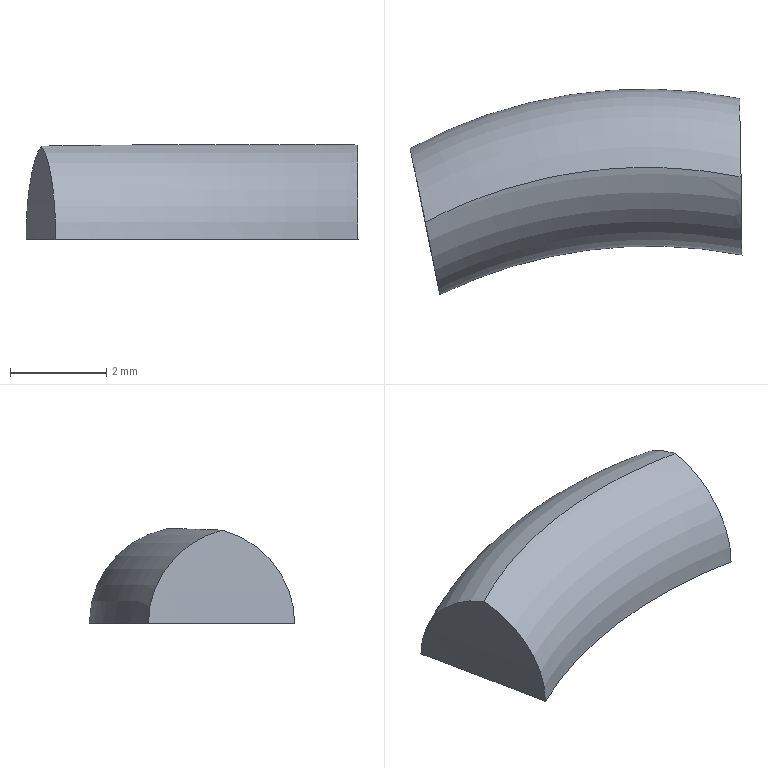Part | STEP file | Twistgrip Indicator Line 3 speed | 1 solid | 5 faces | box 6.882 x 4.262 x 1.965 mm | volume 31.449 mm3 | cylinder 2 | torus 2 | plane 1 | commonest cylinder face diameters 338.024 x1 439.493 x1
STEP:
#1=CARTESIAN_POINT('',(0.,0.,0.));
#2=DIRECTION('',(0.,0.,1.));
#3=DIRECTION('',(1.,0.,0.));
#4=AXIS2_PLACEMENT_3D('',#1,#2,#3);
#5=CARTESIAN_POINT('',(29.808,-30.693,0.));
#6=VERTEX_POINT('',#5);
#7=CARTESIAN_POINT('',(29.86,-33.937,0.));
#8=VERTEX_POINT('',#7);
#9=CARTESIAN_POINT('',(-189.878,-35.84,0.));
#10=DIRECTION('',(0.,0.,-1.));
#11=DIRECTION('',(-1.,0.,0.));
#12=AXIS2_PLACEMENT_3D('',#9,#10,#11);
#13=CIRCLE('',#12,219.746);
#14=CARTESIAN_POINT('',(-189.878,-35.84,2.));
#15=DIRECTION('',(0.,0.,-1.));
#16=DIRECTION('',(1.,0.,0.));
#17=AXIS2_PLACEMENT_3D('',#14,#15,#16);
#18=CYLINDRICAL_SURFACE('',#17,219.746);
#19=CARTESIAN_POINT('',(3.142,2.));
#20=DIRECTION('',(1.,0.));
#21=VECTOR('',#20,1.);
#22=LINE('',#19,#21);
#23=(GEOMETRIC_REPRESENTATION_CONTEXT(2)PARAMETRIC_REPRESENTATION_CONTEXT()REPRESENTATION_CONTEXT('',''));
#24=DEFINITIONAL_REPRESENTATION('',(#22),#23);
#25=PCURVE('',#18,#24);
#26=CARTESIAN_POINT('',(-57.249,-53.811,0.));
#27=DIRECTION('',(0.,0.,-1.));
#28=DIRECTION('',(1.,0.,0.));
#29=AXIS2_PLACEMENT_3D('',#26,#27,#28);
#30=PLANE('',#29);
#31=CARTESIAN_POINT('',(-132.629,-17.97));
#32=DIRECTION('',(-1.,0.));
#33=AXIS2_PLACEMENT_2D('',#31,#32);
#34=CIRCLE('',#33,219.746);
#35=(GEOMETRIC_REPRESENTATION_CONTEXT(2)PARAMETRIC_REPRESENTATION_CONTEXT()REPRESENTATION_CONTEXT('',''));
#36=DEFINITIONAL_REPRESENTATION('',(#34),#35);
#37=PCURVE('',#30,#36);
#38=SURFACE_CURVE('',#13,(#25,#37),.PCURVE_S1.);
#39=EDGE_CURVE('',#6,#8,#38,.T.);
#40=ORIENTED_EDGE('',*,*,#39,.F.);
#41=CARTESIAN_POINT('',(29.84,-32.322,1.957));
#42=VERTEX_POINT('',#41);
#43=CARTESIAN_POINT('',(29.84,-32.322,1.957));
#44=CARTESIAN_POINT('',(29.836,-32.099,1.911));
#45=CARTESIAN_POINT('',(29.832,-31.879,1.827));
#46=CARTESIAN_POINT('',(29.825,-31.486,1.595));
#47=CARTESIAN_POINT('',(29.821,-31.306,1.444));
#48=CARTESIAN_POINT('',(29.815,-31.011,1.095));
#49=CARTESIAN_POINT('',(29.812,-30.893,0.8917));
#50=CARTESIAN_POINT('',(29.809,-30.735,0.4629));
#51=CARTESIAN_POINT('',(29.808,-30.693,0.2319));
#52=CARTESIAN_POINT('',(29.808,-30.693,0.));
#53=B_SPLINE_CURVE_WITH_KNOTS('',3,(#43,#44,#45,#46,#47,#48,#49,#50,#51,#52),.UNSPECIFIED.,.F.,.F.,(4,2,2,2,4),(0.0004297,0.001115,0.001801,0.002486,0.003172),.UNSPECIFIED.);
#54=CARTESIAN_POINT('',(6.267,0.04339));
#55=CARTESIAN_POINT('',(6.267,0.05174));
#56=CARTESIAN_POINT('',(6.267,0.07095));
#57=CARTESIAN_POINT('',(6.266,0.107));
#58=CARTESIAN_POINT('',(6.266,0.1502));
#59=CARTESIAN_POINT('',(6.265,0.2003));
#60=CARTESIAN_POINT('',(6.265,0.257));
#61=CARTESIAN_POINT('',(6.264,0.3202));
#62=CARTESIAN_POINT('',(6.264,0.3903));
#63=CARTESIAN_POINT('',(6.263,0.4667));
#64=CARTESIAN_POINT('',(6.263,0.549));
#65=CARTESIAN_POINT('',(6.262,0.6369));
#66=CARTESIAN_POINT('',(6.262,0.7297));
#67=CARTESIAN_POINT('',(6.262,0.8277));
#68=CARTESIAN_POINT('',(6.261,0.9308));
#69=CARTESIAN_POINT('',(6.261,1.038));
#70=CARTESIAN_POINT('',(6.261,1.15));
#71=CARTESIAN_POINT('',(6.26,1.264));
#72=CARTESIAN_POINT('',(6.26,1.381));
#73=CARTESIAN_POINT('',(6.26,1.501));
#74=CARTESIAN_POINT('',(6.26,1.624));
#75=CARTESIAN_POINT('',(6.26,1.748));
#76=CARTESIAN_POINT('',(6.26,1.874));
#77=CARTESIAN_POINT('',(6.26,1.958));
#78=CARTESIAN_POINT('',(6.26,2.));
#79=B_SPLINE_CURVE_WITH_KNOTS('',3,(#54,#55,#56,#57,#58,#59,#60,#61,#62,#63,#64,#65,#66,#67,#68,#69,#70,#71,#72,#73,#74,#75,#76,#77,#78),.UNSPECIFIED.,.F.,.F.,(4,1,1,1,1,1,1,1,1,1,1,1,1,1,1,1,1,1,1,1,1,1,4),(0.0004297,0.0005543,0.0006789,0.0008036,0.0009282,0.001053,0.001177,0.001302,0.001427,0.001551,0.001676,0.001801,0.001925,0.00205,0.002175,0.002299,0.002424,0.002548,0.002673,0.002798,0.002922,0.003047,0.003172),.QUASI_UNIFORM_KNOTS.);
#80=(GEOMETRIC_REPRESENTATION_CONTEXT(2)PARAMETRIC_REPRESENTATION_CONTEXT()REPRESENTATION_CONTEXT('',''));
#81=DEFINITIONAL_REPRESENTATION('',(#79),#80);
#82=PCURVE('',#18,#81);
#83=CARTESIAN_POINT('',(27.83,-40.695,0.));
#84=DIRECTION('',(0.,0.,-1.));
#85=DIRECTION('',(1.,0.,0.));
#86=AXIS2_PLACEMENT_3D('',#83,#84,#85);
#87=TOROIDAL_SURFACE('',#86,8.196,2.);
#88=CARTESIAN_POINT('',(4.948,4.921));
#89=CARTESIAN_POINT('',(4.947,4.941));
#90=CARTESIAN_POINT('',(4.945,4.982));
#91=CARTESIAN_POINT('',(4.941,5.043));
#92=CARTESIAN_POINT('',(4.938,5.104));
#93=CARTESIAN_POINT('',(4.935,5.165));
#94=CARTESIAN_POINT('',(4.932,5.226));
#95=CARTESIAN_POINT('',(4.929,5.287));
#96=CARTESIAN_POINT('',(4.927,5.348));
#97=CARTESIAN_POINT('',(4.924,5.41));
#98=CARTESIAN_POINT('',(4.922,5.472));
#99=CARTESIAN_POINT('',(4.92,5.534));
#100=CARTESIAN_POINT('',(4.918,5.596));
#101=CARTESIAN_POINT('',(4.916,5.657));
#102=CARTESIAN_POINT('',(4.915,5.719));
#103=CARTESIAN_POINT('',(4.913,5.782));
#104=CARTESIAN_POINT('',(4.912,5.844));
#105=CARTESIAN_POINT('',(4.911,5.907));
#106=CARTESIAN_POINT('',(4.91,5.969));
#107=CARTESIAN_POINT('',(4.909,6.031));
#108=CARTESIAN_POINT('',(4.908,6.094));
#109=CARTESIAN_POINT('',(4.908,6.157));
#110=CARTESIAN_POINT('',(4.908,6.22));
#111=CARTESIAN_POINT('',(4.908,6.262));
#112=CARTESIAN_POINT('',(4.908,6.283));
#113=B_SPLINE_CURVE_WITH_KNOTS('',3,(#88,#89,#90,#91,#92,#93,#94,#95,#96,#97,#98,#99,#100,#101,#102,#103,#104,#105,#106,#107,#108,#109,#110,#111,#112),.UNSPECIFIED.,.F.,.F.,(4,1,1,1,1,1,1,1,1,1,1,1,1,1,1,1,1,1,1,1,1,1,4),(0.0004297,0.0005543,0.0006789,0.0008036,0.0009282,0.001053,0.001177,0.001302,0.001427,0.001551,0.001676,0.001801,0.001925,0.00205,0.002175,0.002299,0.002424,0.002548,0.002673,0.002798,0.002922,0.003047,0.003172),.QUASI_UNIFORM_KNOTS.);
#114=(GEOMETRIC_REPRESENTATION_CONTEXT(2)PARAMETRIC_REPRESENTATION_CONTEXT()REPRESENTATION_CONTEXT('',''));
#115=DEFINITIONAL_REPRESENTATION('',(#113),#114);
#116=PCURVE('',#87,#115);
#117=SURFACE_CURVE('',#53,(#82,#116),.PCURVE_S1.);
#118=EDGE_CURVE('',#42,#6,#117,.T.);
#119=ORIENTED_EDGE('',*,*,#118,.F.);
#120=CARTESIAN_POINT('',(29.86,-33.937,0.));
#121=CARTESIAN_POINT('',(29.86,-33.937,0.2309));
#122=CARTESIAN_POINT('',(29.859,-33.897,0.4558));
#123=CARTESIAN_POINT('',(29.858,-33.739,0.889));
#124=CARTESIAN_POINT('',(29.857,-33.625,1.088));
#125=CARTESIAN_POINT('',(29.854,-33.331,1.441));
#126=CARTESIAN_POINT('',(29.852,-33.156,1.59));
#127=CARTESIAN_POINT('',(29.847,-32.761,1.826));
#128=CARTESIAN_POINT('',(29.843,-32.548,1.91));
#129=CARTESIAN_POINT('',(29.84,-32.322,1.957));
#130=B_SPLINE_CURVE_WITH_KNOTS('',3,(#120,#121,#122,#123,#124,#125,#126,#127,#128,#129),.UNSPECIFIED.,.F.,.F.,(4,2,2,2,4),(0.,0.0006829,0.001366,0.002049,0.002732),.UNSPECIFIED.);
#131=CARTESIAN_POINT('',(6.275,2.));
#132=CARTESIAN_POINT('',(6.275,1.958));
#133=CARTESIAN_POINT('',(6.275,1.874));
#134=CARTESIAN_POINT('',(6.274,1.75));
#135=CARTESIAN_POINT('',(6.274,1.628));
#136=CARTESIAN_POINT('',(6.274,1.506));
#137=CARTESIAN_POINT('',(6.274,1.387));
#138=CARTESIAN_POINT('',(6.274,1.268));
#139=CARTESIAN_POINT('',(6.274,1.154));
#140=CARTESIAN_POINT('',(6.273,1.043));
#141=CARTESIAN_POINT('',(6.273,0.9363));
#142=CARTESIAN_POINT('',(6.273,0.8335));
#143=CARTESIAN_POINT('',(6.272,0.7347));
#144=CARTESIAN_POINT('',(6.272,0.6409));
#145=CARTESIAN_POINT('',(6.272,0.5528));
#146=CARTESIAN_POINT('',(6.271,0.4705));
#147=CARTESIAN_POINT('',(6.271,0.394));
#148=CARTESIAN_POINT('',(6.27,0.3235));
#149=CARTESIAN_POINT('',(6.27,0.2591));
#150=CARTESIAN_POINT('',(6.269,0.2017));
#151=CARTESIAN_POINT('',(6.269,0.1512));
#152=CARTESIAN_POINT('',(6.268,0.1078));
#153=CARTESIAN_POINT('',(6.268,0.0714));
#154=CARTESIAN_POINT('',(6.267,0.05193));
#155=CARTESIAN_POINT('',(6.267,0.04339));
#156=B_SPLINE_CURVE_WITH_KNOTS('',3,(#131,#132,#133,#134,#135,#136,#137,#138,#139,#140,#141,#142,#143,#144,#145,#146,#147,#148,#149,#150,#151,#152,#153,#154,#155),.UNSPECIFIED.,.F.,.F.,(4,1,1,1,1,1,1,1,1,1,1,1,1,1,1,1,1,1,1,1,1,1,4),(0.,0.0001242,0.0002483,0.0003725,0.0004966,0.0006208,0.000745,0.0008691,0.0009933,0.001117,0.001242,0.001366,0.00149,0.001614,0.001738,0.001862,0.001987,0.002111,0.002235,0.002359,0.002483,0.002607,0.002732),.QUASI_UNIFORM_KNOTS.);
#157=(GEOMETRIC_REPRESENTATION_CONTEXT(2)PARAMETRIC_REPRESENTATION_CONTEXT()REPRESENTATION_CONTEXT('',''));
#158=DEFINITIONAL_REPRESENTATION('',(#156),#157);
#159=PCURVE('',#18,#158);
#160=CARTESIAN_POINT('',(27.956,-43.694,0.));
#161=DIRECTION('',(0.,0.,-1.));
#162=DIRECTION('',(1.,0.,0.));
#163=AXIS2_PLACEMENT_3D('',#160,#161,#162);
#164=TOROIDAL_SURFACE('',#163,11.941,2.);
#165=CARTESIAN_POINT('',(4.905,3.142));
#166=CARTESIAN_POINT('',(4.905,3.163));
#167=CARTESIAN_POINT('',(4.905,3.204));
#168=CARTESIAN_POINT('',(4.905,3.267));
#169=CARTESIAN_POINT('',(4.904,3.329));
#170=CARTESIAN_POINT('',(4.904,3.391));
#171=CARTESIAN_POINT('',(4.903,3.453));
#172=CARTESIAN_POINT('',(4.902,3.516));
#173=CARTESIAN_POINT('',(4.901,3.578));
#174=CARTESIAN_POINT('',(4.9,3.64));
#175=CARTESIAN_POINT('',(4.899,3.702));
#176=CARTESIAN_POINT('',(4.898,3.764));
#177=CARTESIAN_POINT('',(4.896,3.826));
#178=CARTESIAN_POINT('',(4.895,3.888));
#179=CARTESIAN_POINT('',(4.893,3.95));
#180=CARTESIAN_POINT('',(4.891,4.011));
#181=CARTESIAN_POINT('',(4.89,4.073));
#182=CARTESIAN_POINT('',(4.888,4.135));
#183=CARTESIAN_POINT('',(4.886,4.197));
#184=CARTESIAN_POINT('',(4.884,4.258));
#185=CARTESIAN_POINT('',(4.882,4.319));
#186=CARTESIAN_POINT('',(4.88,4.381));
#187=CARTESIAN_POINT('',(4.878,4.442));
#188=CARTESIAN_POINT('',(4.877,4.483));
#189=CARTESIAN_POINT('',(4.877,4.504));
#190=B_SPLINE_CURVE_WITH_KNOTS('',3,(#165,#166,#167,#168,#169,#170,#171,#172,#173,#174,#175,#176,#177,#178,#179,#180,#181,#182,#183,#184,#185,#186,#187,#188,#189),.UNSPECIFIED.,.F.,.F.,(4,1,1,1,1,1,1,1,1,1,1,1,1,1,1,1,1,1,1,1,1,1,4),(0.,0.0001242,0.0002483,0.0003725,0.0004966,0.0006208,0.000745,0.0008691,0.0009933,0.001117,0.001242,0.001366,0.00149,0.001614,0.001738,0.001862,0.001987,0.002111,0.002235,0.002359,0.002483,0.002607,0.002732),.QUASI_UNIFORM_KNOTS.);
#191=(GEOMETRIC_REPRESENTATION_CONTEXT(2)PARAMETRIC_REPRESENTATION_CONTEXT()REPRESENTATION_CONTEXT('',''));
#192=DEFINITIONAL_REPRESENTATION('',(#190),#191);
#193=PCURVE('',#164,#192);
#194=SURFACE_CURVE('',#130,(#159,#193),.PCURVE_S1.);
#195=EDGE_CURVE('',#8,#42,#194,.T.);
#196=ORIENTED_EDGE('',*,*,#195,.F.);
#197=EDGE_LOOP('',(#40,#119,#196));
#198=FACE_BOUND('',#197,.T.);
#199=ADVANCED_FACE('',(#198),#18,.T.);
#200=CARTESIAN_POINT('',(23.297,-33.259,1.933));
#201=VERTEX_POINT('',#200);
#202=CARTESIAN_POINT('',(23.595,-34.761,0.));
#203=VERTEX_POINT('',#202);
#204=CARTESIAN_POINT('',(23.297,-33.259,1.933));
#205=CARTESIAN_POINT('',(23.318,-33.363,1.905));
#206=CARTESIAN_POINT('',(23.339,-33.467,1.869));
#207=CARTESIAN_POINT('',(23.379,-33.666,1.78));
#208=CARTESIAN_POINT('',(23.398,-33.761,1.728));
#209=CARTESIAN_POINT('',(23.434,-33.942,1.609));
#210=CARTESIAN_POINT('',(23.452,-34.03,1.542));
#211=CARTESIAN_POINT('',(23.484,-34.191,1.394));
#212=CARTESIAN_POINT('',(23.498,-34.265,1.314));
#213=CARTESIAN_POINT('',(23.538,-34.468,1.057));
#214=CARTESIAN_POINT('',(23.559,-34.577,0.8596));
#215=CARTESIAN_POINT('',(23.588,-34.722,0.4455));
#216=CARTESIAN_POINT('',(23.595,-34.761,0.2232));
#217=CARTESIAN_POINT('',(23.595,-34.761,0.));
#218=B_SPLINE_CURVE_WITH_KNOTS('',3,(#204,#205,#206,#207,#208,#209,#210,#211,#212,#213,#214,#215,#216,#217),.UNSPECIFIED.,.F.,.F.,(4,2,2,2,2,2,4),(0.0005285,0.0008583,0.001188,0.001518,0.001848,0.002507,0.003167),.UNSPECIFIED.);
#219=CARTESIAN_POINT('',(-142.328,-66.926,2.));
#220=DIRECTION('',(0.,0.,-1.));
#221=DIRECTION('',(1.,0.,0.));
#222=AXIS2_PLACEMENT_3D('',#219,#220,#221);
#223=CYLINDRICAL_SURFACE('',#222,169.012);
#224=CARTESIAN_POINT('',(6.083,0.06689));
#225=CARTESIAN_POINT('',(6.083,0.07191));
#226=CARTESIAN_POINT('',(6.083,0.08257));
#227=CARTESIAN_POINT('',(6.083,0.1003));
#228=CARTESIAN_POINT('',(6.084,0.1197));
#229=CARTESIAN_POINT('',(6.084,0.1407));
#230=CARTESIAN_POINT('',(6.084,0.1633));
#231=CARTESIAN_POINT('',(6.085,0.1874));
#232=CARTESIAN_POINT('',(6.085,0.2131));
#233=CARTESIAN_POINT('',(6.085,0.2402));
#234=CARTESIAN_POINT('',(6.086,0.2689));
#235=CARTESIAN_POINT('',(6.086,0.2991));
#236=CARTESIAN_POINT('',(6.086,0.3308));
#237=CARTESIAN_POINT('',(6.087,0.364));
#238=CARTESIAN_POINT('',(6.087,0.3989));
#239=CARTESIAN_POINT('',(6.087,0.4353));
#240=CARTESIAN_POINT('',(6.087,0.4731));
#241=CARTESIAN_POINT('',(6.088,0.5122));
#242=CARTESIAN_POINT('',(6.088,0.5525));
#243=CARTESIAN_POINT('',(6.088,0.594));
#244=CARTESIAN_POINT('',(6.088,0.6367));
#245=CARTESIAN_POINT('',(6.089,0.6805));
#246=CARTESIAN_POINT('',(6.089,0.7255));
#247=CARTESIAN_POINT('',(6.089,0.7717));
#248=CARTESIAN_POINT('',(6.089,0.8191));
#249=CARTESIAN_POINT('',(6.09,0.8677));
#250=CARTESIAN_POINT('',(6.09,0.9174));
#251=CARTESIAN_POINT('',(6.09,0.9682));
#252=CARTESIAN_POINT('',(6.09,1.02));
#253=CARTESIAN_POINT('',(6.09,1.073));
#254=CARTESIAN_POINT('',(6.09,1.126));
#255=CARTESIAN_POINT('',(6.091,1.18));
#256=CARTESIAN_POINT('',(6.091,1.235));
#257=CARTESIAN_POINT('',(6.091,1.291));
#258=CARTESIAN_POINT('',(6.091,1.347));
#259=CARTESIAN_POINT('',(6.091,1.404));
#260=CARTESIAN_POINT('',(6.091,1.462));
#261=CARTESIAN_POINT('',(6.091,1.52));
#262=CARTESIAN_POINT('',(6.091,1.579));
#263=CARTESIAN_POINT('',(6.092,1.638));
#264=CARTESIAN_POINT('',(6.092,1.697));
#265=CARTESIAN_POINT('',(6.092,1.758));
#266=CARTESIAN_POINT('',(6.092,1.818));
#267=CARTESIAN_POINT('',(6.092,1.878));
#268=CARTESIAN_POINT('',(6.092,1.939));
#269=CARTESIAN_POINT('',(6.092,1.98));
#270=CARTESIAN_POINT('',(6.092,2.));
#271=B_SPLINE_CURVE_WITH_KNOTS('',3,(#224,#225,#226,#227,#228,#229,#230,#231,#232,#233,#234,#235,#236,#237,#238,#239,#240,#241,#242,#243,#244,#245,#246,#247,#248,#249,#250,#251,#252,#253,#254,#255,#256,#257,#258,#259,#260,#261,#262,#263,#264,#265,#266,#267,#268,#269,#270),.UNSPECIFIED.,.F.,.F.,(4,1,1,1,1,1,1,1,1,1,1,1,1,1,1,1,1,1,1,1,1,1,1,1,1,1,1,1,1,1,1,1,1,1,1,1,1,1,1,1,1,1,1,1,4),(0.0005285,0.0005885,0.0006485,0.0007084,0.0007684,0.0008283,0.0008883,0.0009482,0.001008,0.001068,0.001128,0.001188,0.001248,0.001308,0.001368,0.001428,0.001488,0.001548,0.001608,0.001668,0.001728,0.001788,0.001848,0.001907,0.001967,0.002027,0.002087,0.002147,0.002207,0.002267,0.002327,0.002387,0.002447,0.002507,0.002567,0.002627,0.002687,0.002747,0.002807,0.002867,0.002927,0.002987,0.003047,0.003107,0.003167),.QUASI_UNIFORM_KNOTS.);
#272=(GEOMETRIC_REPRESENTATION_CONTEXT(2)PARAMETRIC_REPRESENTATION_CONTEXT()REPRESENTATION_CONTEXT('',''));
#273=DEFINITIONAL_REPRESENTATION('',(#271),#272);
#274=PCURVE('',#223,#273);
#275=CARTESIAN_POINT('',(4.293,4.453));
#276=CARTESIAN_POINT('',(4.292,4.443));
#277=CARTESIAN_POINT('',(4.291,4.424));
#278=CARTESIAN_POINT('',(4.29,4.394));
#279=CARTESIAN_POINT('',(4.289,4.364));
#280=CARTESIAN_POINT('',(4.288,4.335));
#281=CARTESIAN_POINT('',(4.287,4.305));
#282=CARTESIAN_POINT('',(4.286,4.276));
#283=CARTESIAN_POINT('',(4.285,4.246));
#284=CARTESIAN_POINT('',(4.284,4.217));
#285=CARTESIAN_POINT('',(4.282,4.188));
#286=CARTESIAN_POINT('',(4.281,4.158));
#287=CARTESIAN_POINT('',(4.28,4.129));
#288=CARTESIAN_POINT('',(4.279,4.099));
#289=CARTESIAN_POINT('',(4.278,4.07));
#290=CARTESIAN_POINT('',(4.277,4.04));
#291=CARTESIAN_POINT('',(4.276,4.01));
#292=CARTESIAN_POINT('',(4.275,3.98));
#293=CARTESIAN_POINT('',(4.274,3.951));
#294=CARTESIAN_POINT('',(4.273,3.921));
#295=CARTESIAN_POINT('',(4.272,3.891));
#296=CARTESIAN_POINT('',(4.271,3.862));
#297=CARTESIAN_POINT('',(4.27,3.832));
#298=CARTESIAN_POINT('',(4.269,3.803));
#299=CARTESIAN_POINT('',(4.268,3.773));
#300=CARTESIAN_POINT('',(4.267,3.743));
#301=CARTESIAN_POINT('',(4.267,3.713));
#302=CARTESIAN_POINT('',(4.266,3.684));
#303=CARTESIAN_POINT('',(4.265,3.654));
#304=CARTESIAN_POINT('',(4.264,3.624));
#305=CARTESIAN_POINT('',(4.264,3.594));
#306=CARTESIAN_POINT('',(4.263,3.564));
#307=CARTESIAN_POINT('',(4.262,3.534));
#308=CARTESIAN_POINT('',(4.262,3.504));
#309=CARTESIAN_POINT('',(4.261,3.474));
#310=CARTESIAN_POINT('',(4.261,3.444));
#311=CARTESIAN_POINT('',(4.26,3.414));
#312=CARTESIAN_POINT('',(4.26,3.384));
#313=CARTESIAN_POINT('',(4.26,3.354));
#314=CARTESIAN_POINT('',(4.259,3.324));
#315=CARTESIAN_POINT('',(4.259,3.293));
#316=CARTESIAN_POINT('',(4.259,3.263));
#317=CARTESIAN_POINT('',(4.259,3.233));
#318=CARTESIAN_POINT('',(4.258,3.202));
#319=CARTESIAN_POINT('',(4.258,3.172));
#320=CARTESIAN_POINT('',(4.258,3.152));
#321=CARTESIAN_POINT('',(4.258,3.142));
#322=B_SPLINE_CURVE_WITH_KNOTS('',3,(#275,#276,#277,#278,#279,#280,#281,#282,#283,#284,#285,#286,#287,#288,#289,#290,#291,#292,#293,#294,#295,#296,#297,#298,#299,#300,#301,#302,#303,#304,#305,#306,#307,#308,#309,#310,#311,#312,#313,#314,#315,#316,#317,#318,#319,#320,#321),.UNSPECIFIED.,.F.,.F.,(4,1,1,1,1,1,1,1,1,1,1,1,1,1,1,1,1,1,1,1,1,1,1,1,1,1,1,1,1,1,1,1,1,1,1,1,1,1,1,1,1,1,1,1,4),(0.0005285,0.0005885,0.0006485,0.0007084,0.0007684,0.0008283,0.0008883,0.0009482,0.001008,0.001068,0.001128,0.001188,0.001248,0.001308,0.001368,0.001428,0.001488,0.001548,0.001608,0.001668,0.001728,0.001788,0.001848,0.001907,0.001967,0.002027,0.002087,0.002147,0.002207,0.002267,0.002327,0.002387,0.002447,0.002507,0.002567,0.002627,0.002687,0.002747,0.002807,0.002867,0.002927,0.002987,0.003047,0.003107,0.003167),.QUASI_UNIFORM_KNOTS.);
#323=(GEOMETRIC_REPRESENTATION_CONTEXT(2)PARAMETRIC_REPRESENTATION_CONTEXT()REPRESENTATION_CONTEXT('',''));
#324=DEFINITIONAL_REPRESENTATION('',(#322),#323);
#325=PCURVE('',#164,#324);
#326=SURFACE_CURVE('',#218,(#274,#325),.PCURVE_S1.);
#327=EDGE_CURVE('',#201,#203,#326,.T.);
#328=ORIENTED_EDGE('',*,*,#327,.T.);
#329=CARTESIAN_POINT('',(22.978,-31.727,0.));
#330=VERTEX_POINT('',#329);
#331=CARTESIAN_POINT('',(-142.328,-66.926,0.));
#332=DIRECTION('',(0.,0.,1.));
#333=DIRECTION('',(-1.,0.,0.));
#334=AXIS2_PLACEMENT_3D('',#331,#332,#333);
#335=CIRCLE('',#334,169.012);
#336=CARTESIAN_POINT('',(9.425,2.));
#337=DIRECTION('',(-1.,0.));
#338=VECTOR('',#337,1.);
#339=LINE('',#336,#338);
#340=(GEOMETRIC_REPRESENTATION_CONTEXT(2)PARAMETRIC_REPRESENTATION_CONTEXT()REPRESENTATION_CONTEXT('',''));
#341=DEFINITIONAL_REPRESENTATION('',(#339),#340);
#342=PCURVE('',#223,#341);
#343=CARTESIAN_POINT('',(-254.091,13.116));
#344=CARTESIAN_POINT('',(-254.091,305.853));
#345=CARTESIAN_POINT('',(-0.5729,159.484));
#346=CARTESIAN_POINT('',(252.945,13.116));
#347=CARTESIAN_POINT('',(-0.5729,-133.253));
#348=CARTESIAN_POINT('',(-254.091,-279.622));
#349=CARTESIAN_POINT('',(-254.091,13.116));
#350=(BOUNDED_CURVE()B_SPLINE_CURVE(2,(#343,#344,#345,#346,#347,#348,#349),.UNSPECIFIED.,.T.,.F.)B_SPLINE_CURVE_WITH_KNOTS((1,2,2,2,2,1),(-2.094,0.,2.094,4.189,6.283,8.378),.UNSPECIFIED.)CURVE()GEOMETRIC_REPRESENTATION_ITEM()RATIONAL_B_SPLINE_CURVE((1.,0.5,1.,0.5,1.,0.5,1.))REPRESENTATION_ITEM(''));
#351=(GEOMETRIC_REPRESENTATION_CONTEXT(2)PARAMETRIC_REPRESENTATION_CONTEXT()REPRESENTATION_CONTEXT('',''));
#352=DEFINITIONAL_REPRESENTATION('',(#350),#351);
#353=PCURVE('',#30,#352);
#354=SURFACE_CURVE('',#335,(#342,#353),.PCURVE_S1.);
#355=EDGE_CURVE('',#203,#330,#354,.T.);
#356=ORIENTED_EDGE('',*,*,#355,.T.);
#357=CARTESIAN_POINT('',(22.978,-31.727,0.));
#358=CARTESIAN_POINT('',(22.978,-31.727,0.2255));
#359=CARTESIAN_POINT('',(22.986,-31.765,0.445));
#360=CARTESIAN_POINT('',(23.018,-31.915,0.8683));
#361=CARTESIAN_POINT('',(23.041,-32.024,1.062));
#362=CARTESIAN_POINT('',(23.1,-32.304,1.409));
#363=CARTESIAN_POINT('',(23.135,-32.469,1.556));
#364=CARTESIAN_POINT('',(23.212,-32.843,1.793));
#365=CARTESIAN_POINT('',(23.253,-33.045,1.879));
#366=CARTESIAN_POINT('',(23.297,-33.259,1.933));
#367=B_SPLINE_CURVE_WITH_KNOTS('',3,(#357,#358,#359,#360,#361,#362,#363,#364,#365,#366),.UNSPECIFIED.,.F.,.F.,(4,2,2,2,4),(0.,0.0006667,0.001333,0.002,0.002667),.UNSPECIFIED.);
#368=CARTESIAN_POINT('',(6.073,2.));
#369=CARTESIAN_POINT('',(6.073,1.959));
#370=CARTESIAN_POINT('',(6.073,1.877));
#371=CARTESIAN_POINT('',(6.073,1.756));
#372=CARTESIAN_POINT('',(6.074,1.636));
#373=CARTESIAN_POINT('',(6.074,1.518));
#374=CARTESIAN_POINT('',(6.074,1.401));
#375=CARTESIAN_POINT('',(6.074,1.285));
#376=CARTESIAN_POINT('',(6.074,1.174));
#377=CARTESIAN_POINT('',(6.075,1.065));
#378=CARTESIAN_POINT('',(6.075,0.9609));
#379=CARTESIAN_POINT('',(6.076,0.8603));
#380=CARTESIAN_POINT('',(6.076,0.7635));
#381=CARTESIAN_POINT('',(6.077,0.6714));
#382=CARTESIAN_POINT('',(6.077,0.5848));
#383=CARTESIAN_POINT('',(6.078,0.5036));
#384=CARTESIAN_POINT('',(6.078,0.4279));
#385=CARTESIAN_POINT('',(6.079,0.3578));
#386=CARTESIAN_POINT('',(6.079,0.2931));
#387=CARTESIAN_POINT('',(6.08,0.235));
#388=CARTESIAN_POINT('',(6.081,0.1832));
#389=CARTESIAN_POINT('',(6.081,0.1378));
#390=CARTESIAN_POINT('',(6.082,0.09867));
#391=CARTESIAN_POINT('',(6.082,0.07679));
#392=CARTESIAN_POINT('',(6.083,0.06689));
#393=B_SPLINE_CURVE_WITH_KNOTS('',3,(#368,#369,#370,#371,#372,#373,#374,#375,#376,#377,#378,#379,#380,#381,#382,#383,#384,#385,#386,#387,#388,#389,#390,#391,#392),.UNSPECIFIED.,.F.,.F.,(4,1,1,1,1,1,1,1,1,1,1,1,1,1,1,1,1,1,1,1,1,1,4),(0.,0.0001212,0.0002425,0.0003637,0.0004849,0.0006061,0.0007274,0.0008486,0.0009698,0.001091,0.001212,0.001333,0.001455,0.001576,0.001697,0.001818,0.00194,0.002061,0.002182,0.002303,0.002425,0.002546,0.002667),.QUASI_UNIFORM_KNOTS.);
#394=(GEOMETRIC_REPRESENTATION_CONTEXT(2)PARAMETRIC_REPRESENTATION_CONTEXT()REPRESENTATION_CONTEXT('',''));
#395=DEFINITIONAL_REPRESENTATION('',(#393),#394);
#396=PCURVE('',#223,#395);
#397=CARTESIAN_POINT('',(4.216,6.283));
#398=CARTESIAN_POINT('',(4.216,6.263));
#399=CARTESIAN_POINT('',(4.216,6.222));
#400=CARTESIAN_POINT('',(4.216,6.161));
#401=CARTESIAN_POINT('',(4.216,6.101));
#402=CARTESIAN_POINT('',(4.215,6.04));
#403=CARTESIAN_POINT('',(4.214,5.979));
#404=CARTESIAN_POINT('',(4.213,5.918));
#405=CARTESIAN_POINT('',(4.211,5.858));
#406=CARTESIAN_POINT('',(4.21,5.797));
#407=CARTESIAN_POINT('',(4.208,5.737));
#408=CARTESIAN_POINT('',(4.206,5.677));
#409=CARTESIAN_POINT('',(4.204,5.617));
#410=CARTESIAN_POINT('',(4.201,5.557));
#411=CARTESIAN_POINT('',(4.198,5.498));
#412=CARTESIAN_POINT('',(4.196,5.439));
#413=CARTESIAN_POINT('',(4.192,5.38));
#414=CARTESIAN_POINT('',(4.189,5.321));
#415=CARTESIAN_POINT('',(4.186,5.262));
#416=CARTESIAN_POINT('',(4.182,5.203));
#417=CARTESIAN_POINT('',(4.178,5.145));
#418=CARTESIAN_POINT('',(4.174,5.087));
#419=CARTESIAN_POINT('',(4.17,5.03));
#420=CARTESIAN_POINT('',(4.167,4.991));
#421=CARTESIAN_POINT('',(4.165,4.972));
#422=B_SPLINE_CURVE_WITH_KNOTS('',3,(#397,#398,#399,#400,#401,#402,#403,#404,#405,#406,#407,#408,#409,#410,#411,#412,#413,#414,#415,#416,#417,#418,#419,#420,#421),.UNSPECIFIED.,.F.,.F.,(4,1,1,1,1,1,1,1,1,1,1,1,1,1,1,1,1,1,1,1,1,1,4),(0.,0.0001212,0.0002425,0.0003637,0.0004849,0.0006061,0.0007274,0.0008486,0.0009698,0.001091,0.001212,0.001333,0.001455,0.001576,0.001697,0.001818,0.00194,0.002061,0.002182,0.002303,0.002425,0.002546,0.002667),.QUASI_UNIFORM_KNOTS.);
#423=(GEOMETRIC_REPRESENTATION_CONTEXT(2)PARAMETRIC_REPRESENTATION_CONTEXT()REPRESENTATION_CONTEXT('',''));
#424=DEFINITIONAL_REPRESENTATION('',(#422),#423);
#425=PCURVE('',#87,#424);
#426=SURFACE_CURVE('',#367,(#396,#425),.PCURVE_S1.);
#427=EDGE_CURVE('',#330,#201,#426,.T.);
#428=ORIENTED_EDGE('',*,*,#427,.T.);
#429=EDGE_LOOP('',(#328,#356,#428));
#430=FACE_BOUND('',#429,.F.);
#431=ADVANCED_FACE('',(#430),#223,.F.);
#432=CARTESIAN_POINT('',(27.83,-40.695,0.));
#433=DIRECTION('',(0.,0.,-1.));
#434=DIRECTION('',(1.,0.,0.));
#435=AXIS2_PLACEMENT_3D('',#432,#433,#434);
#436=CIRCLE('',#435,10.196);
#437=CARTESIAN_POINT('',(85.079,-13.116));
#438=DIRECTION('',(1.,0.));
#439=AXIS2_PLACEMENT_2D('',#437,#438);
#440=CIRCLE('',#439,10.196);
#441=(GEOMETRIC_REPRESENTATION_CONTEXT(2)PARAMETRIC_REPRESENTATION_CONTEXT()REPRESENTATION_CONTEXT('',''));
#442=DEFINITIONAL_REPRESENTATION('',(#440),#441);
#443=PCURVE('',#30,#442);
#444=CARTESIAN_POINT('',(0.,6.283));
#445=DIRECTION('',(1.,0.));
#446=VECTOR('',#445,1.);
#447=LINE('',#444,#446);
#448=(GEOMETRIC_REPRESENTATION_CONTEXT(2)PARAMETRIC_REPRESENTATION_CONTEXT()REPRESENTATION_CONTEXT('',''));
#449=DEFINITIONAL_REPRESENTATION('',(#447),#448);
#450=PCURVE('',#87,#449);
#451=SURFACE_CURVE('',#436,(#443,#450),.PCURVE_S1.);
#452=EDGE_CURVE('',#330,#6,#451,.T.);
#453=ORIENTED_EDGE('',*,*,#452,.T.);
#454=ORIENTED_EDGE('',*,*,#39,.T.);
#455=CARTESIAN_POINT('',(27.956,-43.694,0.));
#456=DIRECTION('',(0.,0.,1.));
#457=DIRECTION('',(1.,0.,0.));
#458=AXIS2_PLACEMENT_3D('',#455,#456,#457);
#459=CIRCLE('',#458,9.941);
#460=CARTESIAN_POINT('',(95.146,-10.116));
#461=CARTESIAN_POINT('',(95.146,-27.335));
#462=CARTESIAN_POINT('',(80.234,-18.726));
#463=CARTESIAN_POINT('',(65.322,-10.116));
#464=CARTESIAN_POINT('',(80.234,-1.507));
#465=CARTESIAN_POINT('',(95.146,7.103));
#466=CARTESIAN_POINT('',(95.146,-10.116));
#467=(BOUNDED_CURVE()B_SPLINE_CURVE(2,(#460,#461,#462,#463,#464,#465,#466),.UNSPECIFIED.,.T.,.F.)B_SPLINE_CURVE_WITH_KNOTS((1,2,2,2,2,1),(-2.094,0.,2.094,4.189,6.283,8.378),.UNSPECIFIED.)CURVE()GEOMETRIC_REPRESENTATION_ITEM()RATIONAL_B_SPLINE_CURVE((1.,0.5,1.,0.5,1.,0.5,1.))REPRESENTATION_ITEM(''));
#468=(GEOMETRIC_REPRESENTATION_CONTEXT(2)PARAMETRIC_REPRESENTATION_CONTEXT()REPRESENTATION_CONTEXT('',''));
#469=DEFINITIONAL_REPRESENTATION('',(#467),#468);
#470=PCURVE('',#30,#469);
#471=CARTESIAN_POINT('',(6.283,3.142));
#472=DIRECTION('',(-1.,0.));
#473=VECTOR('',#472,1.);
#474=LINE('',#471,#473);
#475=(GEOMETRIC_REPRESENTATION_CONTEXT(2)PARAMETRIC_REPRESENTATION_CONTEXT()REPRESENTATION_CONTEXT('',''));
#476=DEFINITIONAL_REPRESENTATION('',(#474),#475);
#477=PCURVE('',#164,#476);
#478=SURFACE_CURVE('',#459,(#470,#477),.PCURVE_S1.);
#479=EDGE_CURVE('',#8,#203,#478,.T.);
#480=ORIENTED_EDGE('',*,*,#479,.T.);
#481=ORIENTED_EDGE('',*,*,#355,.T.);
#482=EDGE_LOOP('',(#453,#454,#480,#481));
#483=FACE_BOUND('',#482,.T.);
#484=ADVANCED_FACE('',(#483),#30,.T.);
#485=ORIENTED_EDGE('',*,*,#452,.F.);
#486=ORIENTED_EDGE('',*,*,#427,.T.);
#487=CARTESIAN_POINT('',(23.297,-33.259,1.933));
#488=CARTESIAN_POINT('',(23.798,-32.996,1.943));
#489=CARTESIAN_POINT('',(24.315,-32.778,1.949));
#490=CARTESIAN_POINT('',(25.114,-32.52,1.957));
#491=CARTESIAN_POINT('',(25.384,-32.445,1.959));
#492=CARTESIAN_POINT('',(25.933,-32.317,1.962));
#493=CARTESIAN_POINT('',(26.212,-32.265,1.963));
#494=CARTESIAN_POINT('',(27.052,-32.145,1.965));
#495=CARTESIAN_POINT('',(27.611,-32.114,1.966));
#496=CARTESIAN_POINT('',(28.727,-32.147,1.963));
#497=CARTESIAN_POINT('',(29.284,-32.21,1.961));
#498=CARTESIAN_POINT('',(29.84,-32.322,1.957));
#499=B_SPLINE_CURVE_WITH_KNOTS('',3,(#487,#488,#489,#490,#491,#492,#493,#494,#495,#496,#497,#498),.UNSPECIFIED.,.F.,.F.,(4,2,2,2,2,4),(0.0001934,0.001873,0.002712,0.003552,0.005231,0.00691),.UNSPECIFIED.);
#500=CARTESIAN_POINT('',(4.165,4.972));
#501=CARTESIAN_POINT('',(4.177,4.968));
#502=CARTESIAN_POINT('',(4.2,4.962));
#503=CARTESIAN_POINT('',(4.236,4.953));
#504=CARTESIAN_POINT('',(4.271,4.944));
#505=CARTESIAN_POINT('',(4.306,4.937));
#506=CARTESIAN_POINT('',(4.341,4.93));
#507=CARTESIAN_POINT('',(4.377,4.924));
#508=CARTESIAN_POINT('',(4.412,4.918));
#509=CARTESIAN_POINT('',(4.448,4.913));
#510=CARTESIAN_POINT('',(4.484,4.909));
#511=CARTESIAN_POINT('',(4.52,4.906));
#512=CARTESIAN_POINT('',(4.556,4.903));
#513=CARTESIAN_POINT('',(4.592,4.901));
#514=CARTESIAN_POINT('',(4.627,4.9));
#515=CARTESIAN_POINT('',(4.663,4.899));
#516=CARTESIAN_POINT('',(4.699,4.899));
#517=CARTESIAN_POINT('',(4.734,4.9));
#518=CARTESIAN_POINT('',(4.77,4.902));
#519=CARTESIAN_POINT('',(4.805,4.904));
#520=CARTESIAN_POINT('',(4.841,4.907));
#521=CARTESIAN_POINT('',(4.876,4.911));
#522=CARTESIAN_POINT('',(4.912,4.916));
#523=CARTESIAN_POINT('',(4.936,4.919));
#524=CARTESIAN_POINT('',(4.948,4.921));
#525=B_SPLINE_CURVE_WITH_KNOTS('',3,(#500,#501,#502,#503,#504,#505,#506,#507,#508,#509,#510,#511,#512,#513,#514,#515,#516,#517,#518,#519,#520,#521,#522,#523,#524),.UNSPECIFIED.,.F.,.F.,(4,1,1,1,1,1,1,1,1,1,1,1,1,1,1,1,1,1,1,1,1,1,4),(0.0001934,0.0004987,0.000804,0.001109,0.001415,0.00172,0.002025,0.002331,0.002636,0.002941,0.003246,0.003552,0.003857,0.004162,0.004468,0.004773,0.005078,0.005384,0.005689,0.005994,0.0063,0.006605,0.00691),.QUASI_UNIFORM_KNOTS.);
#526=(GEOMETRIC_REPRESENTATION_CONTEXT(2)PARAMETRIC_REPRESENTATION_CONTEXT()REPRESENTATION_CONTEXT('',''));
#527=DEFINITIONAL_REPRESENTATION('',(#525),#526);
#528=PCURVE('',#87,#527);
#529=CARTESIAN_POINT('',(4.293,4.453));
#530=CARTESIAN_POINT('',(4.301,4.456));
#531=CARTESIAN_POINT('',(4.319,4.463));
#532=CARTESIAN_POINT('',(4.346,4.472));
#533=CARTESIAN_POINT('',(4.373,4.48));
#534=CARTESIAN_POINT('',(4.399,4.488));
#535=CARTESIAN_POINT('',(4.426,4.495));
#536=CARTESIAN_POINT('',(4.452,4.501));
#537=CARTESIAN_POINT('',(4.479,4.507));
#538=CARTESIAN_POINT('',(4.505,4.512));
#539=CARTESIAN_POINT('',(4.532,4.516));
#540=CARTESIAN_POINT('',(4.559,4.519));
#541=CARTESIAN_POINT('',(4.585,4.522));
#542=CARTESIAN_POINT('',(4.612,4.524));
#543=CARTESIAN_POINT('',(4.639,4.525));
#544=CARTESIAN_POINT('',(4.665,4.526));
#545=CARTESIAN_POINT('',(4.691,4.525));
#546=CARTESIAN_POINT('',(4.718,4.524));
#547=CARTESIAN_POINT('',(4.744,4.523));
#548=CARTESIAN_POINT('',(4.77,4.521));
#549=CARTESIAN_POINT('',(4.797,4.517));
#550=CARTESIAN_POINT('',(4.823,4.514));
#551=CARTESIAN_POINT('',(4.85,4.509));
#552=CARTESIAN_POINT('',(4.868,4.506));
#553=CARTESIAN_POINT('',(4.877,4.504));
#554=B_SPLINE_CURVE_WITH_KNOTS('',3,(#529,#530,#531,#532,#533,#534,#535,#536,#537,#538,#539,#540,#541,#542,#543,#544,#545,#546,#547,#548,#549,#550,#551,#552,#553),.UNSPECIFIED.,.F.,.F.,(4,1,1,1,1,1,1,1,1,1,1,1,1,1,1,1,1,1,1,1,1,1,4),(0.0001934,0.0004987,0.000804,0.001109,0.001415,0.00172,0.002025,0.002331,0.002636,0.002941,0.003246,0.003552,0.003857,0.004162,0.004468,0.004773,0.005078,0.005384,0.005689,0.005994,0.0063,0.006605,0.00691),.QUASI_UNIFORM_KNOTS.);
#555=(GEOMETRIC_REPRESENTATION_CONTEXT(2)PARAMETRIC_REPRESENTATION_CONTEXT()REPRESENTATION_CONTEXT('',''));
#556=DEFINITIONAL_REPRESENTATION('',(#554),#555);
#557=PCURVE('',#164,#556);
#558=SURFACE_CURVE('',#499,(#528,#557),.PCURVE_S1.);
#559=EDGE_CURVE('',#201,#42,#558,.T.);
#560=ORIENTED_EDGE('',*,*,#559,.T.);
#561=ORIENTED_EDGE('',*,*,#118,.T.);
#562=EDGE_LOOP('',(#485,#486,#560,#561));
#563=FACE_BOUND('',#562,.T.);
#564=ADVANCED_FACE('',(#563),#87,.T.);
#565=ORIENTED_EDGE('',*,*,#195,.T.);
#566=ORIENTED_EDGE('',*,*,#559,.F.);
#567=ORIENTED_EDGE('',*,*,#327,.T.);
#568=ORIENTED_EDGE('',*,*,#479,.F.);
#569=EDGE_LOOP('',(#565,#566,#567,#568));
#570=FACE_BOUND('',#569,.T.);
#571=ADVANCED_FACE('',(#570),#164,.T.);
#572=CLOSED_SHELL('',(#199,#431,#484,#564,#571));
#573=MANIFOLD_SOLID_BREP('',#572);
#574=(LENGTH_UNIT()NAMED_UNIT(*)SI_UNIT(.MILLI.,.METRE.));
#575=UNCERTAINTY_MEASURE_WITH_UNIT(LENGTH_MEASURE(0.0002),#574,'','');
#576=(NAMED_UNIT(*)PLANE_ANGLE_UNIT()SI_UNIT($,.RADIAN.));
#577=(NAMED_UNIT(*)SI_UNIT($,.STERADIAN.)SOLID_ANGLE_UNIT());
#578=(GEOMETRIC_REPRESENTATION_CONTEXT(3)GLOBAL_UNCERTAINTY_ASSIGNED_CONTEXT((#575))GLOBAL_UNIT_ASSIGNED_CONTEXT((#574,#576,#577))REPRESENTATION_CONTEXT('',''));
#579=ADVANCED_BREP_SHAPE_REPRESENTATION('',(#4,#573),#578);